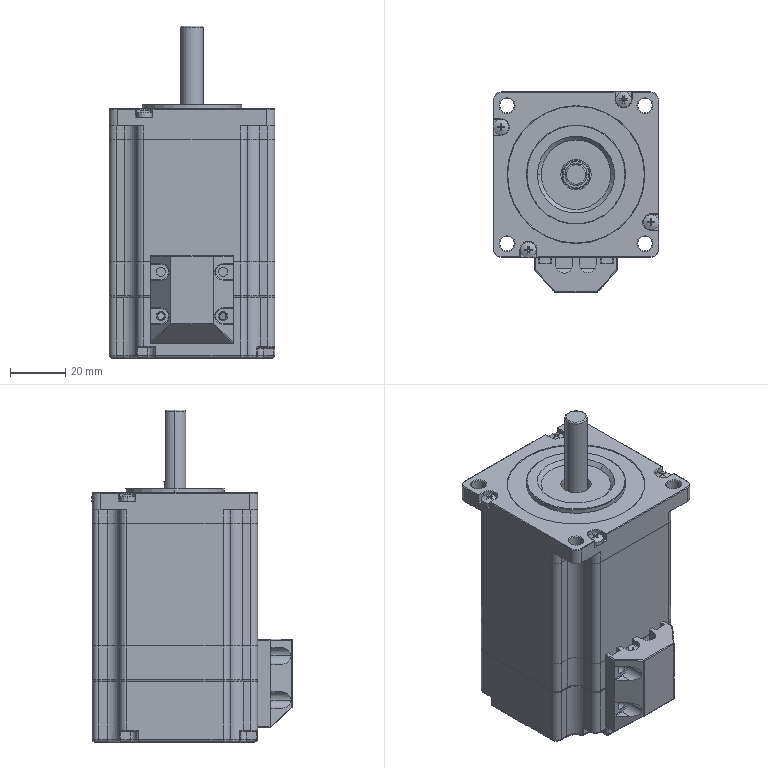Part | 10 solids | 2597 faces | box 60.1 x 72.55 x 120.3 mm | volume 164533 mm3 | cone 1937 | plane 307 | cylinder 271 | spline 82 | commonest cylinder face diameters 0.6 x42 5 x32 1 x30 2 x16 3.2 x16 9 x14